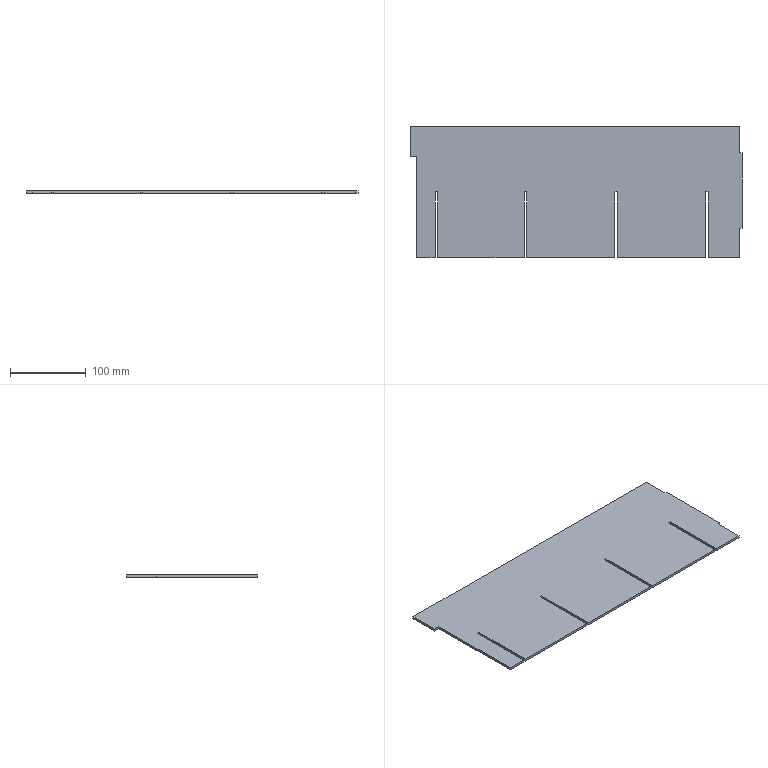Part | SolidWorks | features FlatPattern 1, SMBaseFlange 1, SheetMetal 1 | 1 solid | 28 faces | box 439 x 173.7 x 3.2 mm | volume 236184 mm3 | plane 28
STEP:
#1=CARTESIAN_POINT('',(-218.,59.63,0.));
#2=VERTEX_POINT('',#1);
#3=CARTESIAN_POINT('',(-654.,59.63,0.));
#4=VERTEX_POINT('',#3);
#5=CARTESIAN_POINT('',(-218.,59.63,0.));
#6=DIRECTION('',(-1.,0.,0.));
#7=VECTOR('',#6,1000.);
#8=LINE('',#5,#7);
#9=EDGE_CURVE('',#2,#4,#8,.T.);
#10=ORIENTED_EDGE('',*,*,#9,.T.);
#11=CARTESIAN_POINT('',(-654.,59.63,3.2));
#12=VERTEX_POINT('',#11);
#13=CARTESIAN_POINT('',(-654.,59.63,3.2));
#14=DIRECTION('',(0.,0.,-1.));
#15=VECTOR('',#14,1000.);
#16=LINE('',#13,#15);
#17=EDGE_CURVE('',#12,#4,#16,.T.);
#18=ORIENTED_EDGE('',*,*,#17,.F.);
#19=CARTESIAN_POINT('',(-218.,59.63,3.2));
#20=VERTEX_POINT('',#19);
#21=CARTESIAN_POINT('',(-218.,59.63,3.2));
#22=DIRECTION('',(-1.,0.,0.));
#23=VECTOR('',#22,1000.);
#24=LINE('',#21,#23);
#25=EDGE_CURVE('',#20,#12,#24,.T.);
#26=ORIENTED_EDGE('',*,*,#25,.F.);
#27=CARTESIAN_POINT('',(-218.,59.63,3.2));
#28=DIRECTION('',(0.,0.,-1.));
#29=VECTOR('',#28,1000.);
#30=LINE('',#27,#29);
#31=EDGE_CURVE('',#20,#2,#30,.T.);
#32=ORIENTED_EDGE('',*,*,#31,.T.);
#33=EDGE_LOOP('',(#10,#18,#26,#32));
#34=FACE_OUTER_BOUND('',#33,.T.);
#35=CARTESIAN_POINT('',(-218.,59.63,3.2));
#36=DIRECTION('',(0.,-1.,0.));
#37=DIRECTION('',(0.,0.,-1.));
#38=AXIS2_PLACEMENT_3D('',#35,#36,#37);
#39=PLANE('',#38);
#40=ADVANCED_FACE('',(#34),#39,.F.);
#41=CARTESIAN_POINT('',(-654.,19.93,0.));
#42=VERTEX_POINT('',#41);
#43=CARTESIAN_POINT('',(-654.,59.63,0.));
#44=DIRECTION('',(0.,-1.,0.));
#45=VECTOR('',#44,1000.);
#46=LINE('',#43,#45);
#47=EDGE_CURVE('',#4,#42,#46,.T.);
#48=ORIENTED_EDGE('',*,*,#47,.T.);
#49=CARTESIAN_POINT('',(-654.,19.93,3.2));
#50=VERTEX_POINT('',#49);
#51=CARTESIAN_POINT('',(-654.,19.93,3.2));
#52=DIRECTION('',(0.,0.,-1.));
#53=VECTOR('',#52,1000.);
#54=LINE('',#51,#53);
#55=EDGE_CURVE('',#50,#42,#54,.T.);
#56=ORIENTED_EDGE('',*,*,#55,.F.);
#57=CARTESIAN_POINT('',(-654.,59.63,3.2));
#58=DIRECTION('',(0.,-1.,0.));
#59=VECTOR('',#58,1000.);
#60=LINE('',#57,#59);
#61=EDGE_CURVE('',#12,#50,#60,.T.);
#62=ORIENTED_EDGE('',*,*,#61,.F.);
#63=ORIENTED_EDGE('',*,*,#17,.T.);
#64=EDGE_LOOP('',(#48,#56,#62,#63));
#65=FACE_OUTER_BOUND('',#64,.T.);
#66=CARTESIAN_POINT('',(-654.,59.63,3.2));
#67=DIRECTION('',(1.,0.,0.));
#68=DIRECTION('',(0.,0.,-1.));
#69=AXIS2_PLACEMENT_3D('',#66,#67,#68);
#70=PLANE('',#69);
#71=ADVANCED_FACE('',(#65),#70,.F.);
#72=CARTESIAN_POINT('',(-645.7,19.93,0.));
#73=VERTEX_POINT('',#72);
#74=CARTESIAN_POINT('',(-654.,19.93,0.));
#75=DIRECTION('',(1.,0.,0.));
#76=VECTOR('',#75,1000.);
#77=LINE('',#74,#76);
#78=EDGE_CURVE('',#42,#73,#77,.T.);
#79=ORIENTED_EDGE('',*,*,#78,.T.);
#80=CARTESIAN_POINT('',(-645.7,19.93,3.2));
#81=VERTEX_POINT('',#80);
#82=CARTESIAN_POINT('',(-645.7,19.93,3.2));
#83=DIRECTION('',(0.,0.,-1.));
#84=VECTOR('',#83,1000.);
#85=LINE('',#82,#84);
#86=EDGE_CURVE('',#81,#73,#85,.T.);
#87=ORIENTED_EDGE('',*,*,#86,.F.);
#88=CARTESIAN_POINT('',(-654.,19.93,3.2));
#89=DIRECTION('',(1.,0.,0.));
#90=VECTOR('',#89,1000.);
#91=LINE('',#88,#90);
#92=EDGE_CURVE('',#50,#81,#91,.T.);
#93=ORIENTED_EDGE('',*,*,#92,.F.);
#94=ORIENTED_EDGE('',*,*,#55,.T.);
#95=EDGE_LOOP('',(#79,#87,#93,#94));
#96=FACE_OUTER_BOUND('',#95,.T.);
#97=CARTESIAN_POINT('',(-654.,19.93,3.2));
#98=DIRECTION('',(0.,1.,0.));
#99=DIRECTION('',(0.,0.,1.));
#100=AXIS2_PLACEMENT_3D('',#97,#98,#99);
#101=PLANE('',#100);
#102=ADVANCED_FACE('',(#96),#101,.F.);
#103=CARTESIAN_POINT('',(-645.7,-114.07,0.));
#104=VERTEX_POINT('',#103);
#105=CARTESIAN_POINT('',(-645.7,19.93,0.));
#106=DIRECTION('',(0.,-1.,0.));
#107=VECTOR('',#106,1000.);
#108=LINE('',#105,#107);
#109=EDGE_CURVE('',#73,#104,#108,.T.);
#110=ORIENTED_EDGE('',*,*,#109,.T.);
#111=CARTESIAN_POINT('',(-645.7,-114.07,3.2));
#112=VERTEX_POINT('',#111);
#113=CARTESIAN_POINT('',(-645.7,-114.07,3.2));
#114=DIRECTION('',(0.,0.,-1.));
#115=VECTOR('',#114,1000.);
#116=LINE('',#113,#115);
#117=EDGE_CURVE('',#112,#104,#116,.T.);
#118=ORIENTED_EDGE('',*,*,#117,.F.);
#119=CARTESIAN_POINT('',(-645.7,19.93,3.2));
#120=DIRECTION('',(0.,-1.,0.));
#121=VECTOR('',#120,1000.);
#122=LINE('',#119,#121);
#123=EDGE_CURVE('',#81,#112,#122,.T.);
#124=ORIENTED_EDGE('',*,*,#123,.F.);
#125=ORIENTED_EDGE('',*,*,#86,.T.);
#126=EDGE_LOOP('',(#110,#118,#124,#125));
#127=FACE_OUTER_BOUND('',#126,.T.);
#128=CARTESIAN_POINT('',(-645.7,19.93,3.2));
#129=DIRECTION('',(1.,0.,0.));
#130=DIRECTION('',(0.,1.,0.));
#131=AXIS2_PLACEMENT_3D('',#128,#129,#130);
#132=PLANE('',#131);
#133=ADVANCED_FACE('',(#127),#132,.F.);
#134=CARTESIAN_POINT('',(-620.7,-114.07,0.));
#135=VERTEX_POINT('',#134);
#136=CARTESIAN_POINT('',(-645.7,-114.07,0.));
#137=DIRECTION('',(1.,0.,0.));
#138=VECTOR('',#137,1000.);
#139=LINE('',#136,#138);
#140=EDGE_CURVE('',#104,#135,#139,.T.);
#141=ORIENTED_EDGE('',*,*,#140,.T.);
#142=CARTESIAN_POINT('',(-620.7,-114.07,3.2));
#143=VERTEX_POINT('',#142);
#144=CARTESIAN_POINT('',(-620.7,-114.07,3.2));
#145=DIRECTION('',(0.,0.,-1.));
#146=VECTOR('',#145,1000.);
#147=LINE('',#144,#146);
#148=EDGE_CURVE('',#143,#135,#147,.T.);
#149=ORIENTED_EDGE('',*,*,#148,.F.);
#150=CARTESIAN_POINT('',(-645.7,-114.07,3.2));
#151=DIRECTION('',(1.,0.,0.));
#152=VECTOR('',#151,1000.);
#153=LINE('',#150,#152);
#154=EDGE_CURVE('',#112,#143,#153,.T.);
#155=ORIENTED_EDGE('',*,*,#154,.F.);
#156=ORIENTED_EDGE('',*,*,#117,.T.);
#157=EDGE_LOOP('',(#141,#149,#155,#156));
#158=FACE_OUTER_BOUND('',#157,.T.);
#159=CARTESIAN_POINT('',(-645.7,-114.07,3.2));
#160=DIRECTION('',(0.,1.,0.));
#161=DIRECTION('',(-1.,0.,0.));
#162=AXIS2_PLACEMENT_3D('',#159,#160,#161);
#163=PLANE('',#162);
#164=ADVANCED_FACE('',(#158),#163,.F.);
#165=CARTESIAN_POINT('',(-620.7,-27.07,0.));
#166=VERTEX_POINT('',#165);
#167=CARTESIAN_POINT('',(-620.7,-114.07,0.));
#168=DIRECTION('',(0.,1.,0.));
#169=VECTOR('',#168,1000.);
#170=LINE('',#167,#169);
#171=EDGE_CURVE('',#135,#166,#170,.T.);
#172=ORIENTED_EDGE('',*,*,#171,.T.);
#173=CARTESIAN_POINT('',(-620.7,-27.07,3.2));
#174=VERTEX_POINT('',#173);
#175=CARTESIAN_POINT('',(-620.7,-27.07,3.2));
#176=DIRECTION('',(0.,0.,-1.));
#177=VECTOR('',#176,1000.);
#178=LINE('',#175,#177);
#179=EDGE_CURVE('',#174,#166,#178,.T.);
#180=ORIENTED_EDGE('',*,*,#179,.F.);
#181=CARTESIAN_POINT('',(-620.7,-114.07,3.2));
#182=DIRECTION('',(0.,1.,0.));
#183=VECTOR('',#182,1000.);
#184=LINE('',#181,#183);
#185=EDGE_CURVE('',#143,#174,#184,.T.);
#186=ORIENTED_EDGE('',*,*,#185,.F.);
#187=ORIENTED_EDGE('',*,*,#148,.T.);
#188=EDGE_LOOP('',(#172,#180,#186,#187));
#189=FACE_OUTER_BOUND('',#188,.T.);
#190=CARTESIAN_POINT('',(-620.7,-114.07,3.2));
#191=DIRECTION('',(-1.,0.,0.));
#192=DIRECTION('',(0.,-1.,0.));
#193=AXIS2_PLACEMENT_3D('',#190,#191,#192);
#194=PLANE('',#193);
#195=ADVANCED_FACE('',(#189),#194,.F.);
#196=CARTESIAN_POINT('',(-617.5,-27.07,0.));
#197=VERTEX_POINT('',#196);
#198=CARTESIAN_POINT('',(-620.7,-27.07,0.));
#199=DIRECTION('',(1.,0.,0.));
#200=VECTOR('',#199,1000.);
#201=LINE('',#198,#200);
#202=EDGE_CURVE('',#166,#197,#201,.T.);
#203=ORIENTED_EDGE('',*,*,#202,.T.);
#204=CARTESIAN_POINT('',(-617.5,-27.07,3.2));
#205=VERTEX_POINT('',#204);
#206=CARTESIAN_POINT('',(-617.5,-27.07,3.2));
#207=DIRECTION('',(0.,0.,-1.));
#208=VECTOR('',#207,1000.);
#209=LINE('',#206,#208);
#210=EDGE_CURVE('',#205,#197,#209,.T.);
#211=ORIENTED_EDGE('',*,*,#210,.F.);
#212=CARTESIAN_POINT('',(-620.7,-27.07,3.2));
#213=DIRECTION('',(1.,0.,0.));
#214=VECTOR('',#213,1000.);
#215=LINE('',#212,#214);
#216=EDGE_CURVE('',#174,#205,#215,.T.);
#217=ORIENTED_EDGE('',*,*,#216,.F.);
#218=ORIENTED_EDGE('',*,*,#179,.T.);
#219=EDGE_LOOP('',(#203,#211,#217,#218));
#220=FACE_OUTER_BOUND('',#219,.T.);
#221=CARTESIAN_POINT('',(-620.7,-27.07,3.2));
#222=DIRECTION('',(0.,1.,0.));
#223=DIRECTION('',(0.,0.,1.));
#224=AXIS2_PLACEMENT_3D('',#221,#222,#223);
#225=PLANE('',#224);
#226=ADVANCED_FACE('',(#220),#225,.F.);
#227=CARTESIAN_POINT('',(-617.5,-114.07,0.));
#228=VERTEX_POINT('',#227);
#229=CARTESIAN_POINT('',(-617.5,-27.07,0.));
#230=DIRECTION('',(0.,-1.,0.));
#231=VECTOR('',#230,1000.);
#232=LINE('',#229,#231);
#233=EDGE_CURVE('',#197,#228,#232,.T.);
#234=ORIENTED_EDGE('',*,*,#233,.T.);
#235=CARTESIAN_POINT('',(-617.5,-114.07,3.2));
#236=VERTEX_POINT('',#235);
#237=CARTESIAN_POINT('',(-617.5,-114.07,3.2));
#238=DIRECTION('',(0.,0.,-1.));
#239=VECTOR('',#238,1000.);
#240=LINE('',#237,#239);
#241=EDGE_CURVE('',#236,#228,#240,.T.);
#242=ORIENTED_EDGE('',*,*,#241,.F.);
#243=CARTESIAN_POINT('',(-617.5,-27.07,3.2));
#244=DIRECTION('',(0.,-1.,0.));
#245=VECTOR('',#244,1000.);
#246=LINE('',#243,#245);
#247=EDGE_CURVE('',#205,#236,#246,.T.);
#248=ORIENTED_EDGE('',*,*,#247,.F.);
#249=ORIENTED_EDGE('',*,*,#210,.T.);
#250=EDGE_LOOP('',(#234,#242,#248,#249));
#251=FACE_OUTER_BOUND('',#250,.T.);
#252=CARTESIAN_POINT('',(-617.5,-27.07,3.2));
#253=DIRECTION('',(1.,0.,0.));
#254=DIRECTION('',(0.,1.,0.));
#255=AXIS2_PLACEMENT_3D('',#252,#253,#254);
#256=PLANE('',#255);
#257=ADVANCED_FACE('',(#251),#256,.F.);
#258=CARTESIAN_POINT('',(-503.,-114.07,0.));
#259=VERTEX_POINT('',#258);
#260=CARTESIAN_POINT('',(-617.5,-114.07,0.));
#261=DIRECTION('',(1.,0.,0.));
#262=VECTOR('',#261,1000.);
#263=LINE('',#260,#262);
#264=EDGE_CURVE('',#228,#259,#263,.T.);
#265=ORIENTED_EDGE('',*,*,#264,.T.);
#266=CARTESIAN_POINT('',(-503.,-114.07,3.2));
#267=VERTEX_POINT('',#266);
#268=CARTESIAN_POINT('',(-503.,-114.07,3.2));
#269=DIRECTION('',(0.,0.,-1.));
#270=VECTOR('',#269,1000.);
#271=LINE('',#268,#270);
#272=EDGE_CURVE('',#267,#259,#271,.T.);
#273=ORIENTED_EDGE('',*,*,#272,.F.);
#274=CARTESIAN_POINT('',(-617.5,-114.07,3.2));
#275=DIRECTION('',(1.,0.,0.));
#276=VECTOR('',#275,1000.);
#277=LINE('',#274,#276);
#278=EDGE_CURVE('',#236,#267,#277,.T.);
#279=ORIENTED_EDGE('',*,*,#278,.F.);
#280=ORIENTED_EDGE('',*,*,#241,.T.);
#281=EDGE_LOOP('',(#265,#273,#279,#280));
#282=FACE_OUTER_BOUND('',#281,.T.);
#283=CARTESIAN_POINT('',(-617.5,-114.07,3.2));
#284=DIRECTION('',(0.,1.,0.));
#285=DIRECTION('',(0.,0.,1.));
#286=AXIS2_PLACEMENT_3D('',#283,#284,#285);
#287=PLANE('',#286);
#288=ADVANCED_FACE('',(#282),#287,.F.);
#289=CARTESIAN_POINT('',(-503.,-27.07,0.));
#290=VERTEX_POINT('',#289);
#291=CARTESIAN_POINT('',(-503.,-114.07,0.));
#292=DIRECTION('',(0.,1.,0.));
#293=VECTOR('',#292,1000.);
#294=LINE('',#291,#293);
#295=EDGE_CURVE('',#259,#290,#294,.T.);
#296=ORIENTED_EDGE('',*,*,#295,.T.);
#297=CARTESIAN_POINT('',(-503.,-27.07,3.2));
#298=VERTEX_POINT('',#297);
#299=CARTESIAN_POINT('',(-503.,-27.07,3.2));
#300=DIRECTION('',(0.,0.,-1.));
#301=VECTOR('',#300,1000.);
#302=LINE('',#299,#301);
#303=EDGE_CURVE('',#298,#290,#302,.T.);
#304=ORIENTED_EDGE('',*,*,#303,.F.);
#305=CARTESIAN_POINT('',(-503.,-114.07,3.2));
#306=DIRECTION('',(0.,1.,0.));
#307=VECTOR('',#306,1000.);
#308=LINE('',#305,#307);
#309=EDGE_CURVE('',#267,#298,#308,.T.);
#310=ORIENTED_EDGE('',*,*,#309,.F.);
#311=ORIENTED_EDGE('',*,*,#272,.T.);
#312=EDGE_LOOP('',(#296,#304,#310,#311));
#313=FACE_OUTER_BOUND('',#312,.T.);
#314=CARTESIAN_POINT('',(-503.,-114.07,3.2));
#315=DIRECTION('',(-1.,0.,0.));
#316=DIRECTION('',(0.,0.,1.));
#317=AXIS2_PLACEMENT_3D('',#314,#315,#316);
#318=PLANE('',#317);
#319=ADVANCED_FACE('',(#313),#318,.F.);
#320=CARTESIAN_POINT('',(-499.8,-27.07,0.));
#321=VERTEX_POINT('',#320);
#322=CARTESIAN_POINT('',(-503.,-27.07,0.));
#323=DIRECTION('',(1.,0.,0.));
#324=VECTOR('',#323,1000.);
#325=LINE('',#322,#324);
#326=EDGE_CURVE('',#290,#321,#325,.T.);
#327=ORIENTED_EDGE('',*,*,#326,.T.);
#328=CARTESIAN_POINT('',(-499.8,-27.07,3.2));
#329=VERTEX_POINT('',#328);
#330=CARTESIAN_POINT('',(-499.8,-27.07,3.2));
#331=DIRECTION('',(0.,0.,-1.));
#332=VECTOR('',#331,1000.);
#333=LINE('',#330,#332);
#334=EDGE_CURVE('',#329,#321,#333,.T.);
#335=ORIENTED_EDGE('',*,*,#334,.F.);
#336=CARTESIAN_POINT('',(-503.,-27.07,3.2));
#337=DIRECTION('',(1.,0.,0.));
#338=VECTOR('',#337,1000.);
#339=LINE('',#336,#338);
#340=EDGE_CURVE('',#298,#329,#339,.T.);
#341=ORIENTED_EDGE('',*,*,#340,.F.);
#342=ORIENTED_EDGE('',*,*,#303,.T.);
#343=EDGE_LOOP('',(#327,#335,#341,#342));
#344=FACE_OUTER_BOUND('',#343,.T.);
#345=CARTESIAN_POINT('',(-503.,-27.07,3.2));
#346=DIRECTION('',(0.,1.,0.));
#347=DIRECTION('',(0.,0.,1.));
#348=AXIS2_PLACEMENT_3D('',#345,#346,#347);
#349=PLANE('',#348);
#350=ADVANCED_FACE('',(#344),#349,.F.);
#351=CARTESIAN_POINT('',(-499.8,-114.07,0.));
#352=VERTEX_POINT('',#351);
#353=CARTESIAN_POINT('',(-499.8,-27.07,0.));
#354=DIRECTION('',(0.,-1.,0.));
#355=VECTOR('',#354,1000.);
#356=LINE('',#353,#355);
#357=EDGE_CURVE('',#321,#352,#356,.T.);
#358=ORIENTED_EDGE('',*,*,#357,.T.);
#359=CARTESIAN_POINT('',(-499.8,-114.07,3.2));
#360=VERTEX_POINT('',#359);
#361=CARTESIAN_POINT('',(-499.8,-114.07,3.2));
#362=DIRECTION('',(0.,0.,-1.));
#363=VECTOR('',#362,1000.);
#364=LINE('',#361,#363);
#365=EDGE_CURVE('',#360,#352,#364,.T.);
#366=ORIENTED_EDGE('',*,*,#365,.F.);
#367=CARTESIAN_POINT('',(-499.8,-27.07,3.2));
#368=DIRECTION('',(0.,-1.,0.));
#369=VECTOR('',#368,1000.);
#370=LINE('',#367,#369);
#371=EDGE_CURVE('',#329,#360,#370,.T.);
#372=ORIENTED_EDGE('',*,*,#371,.F.);
#373=ORIENTED_EDGE('',*,*,#334,.T.);
#374=EDGE_LOOP('',(#358,#366,#372,#373));
#375=FACE_OUTER_BOUND('',#374,.T.);
#376=CARTESIAN_POINT('',(-499.8,-27.07,3.2));
#377=DIRECTION('',(1.,0.,0.));
#378=DIRECTION('',(0.,0.,-1.));
#379=AXIS2_PLACEMENT_3D('',#376,#377,#378);
#380=PLANE('',#379);
#381=ADVANCED_FACE('',(#375),#380,.F.);
#382=CARTESIAN_POINT('',(-383.,-114.07,0.));
#383=VERTEX_POINT('',#382);
#384=CARTESIAN_POINT('',(-499.8,-114.07,0.));
#385=DIRECTION('',(1.,0.,0.));
#386=VECTOR('',#385,1000.);
#387=LINE('',#384,#386);
#388=EDGE_CURVE('',#352,#383,#387,.T.);
#389=ORIENTED_EDGE('',*,*,#388,.T.);
#390=CARTESIAN_POINT('',(-383.,-114.07,3.2));
#391=VERTEX_POINT('',#390);
#392=CARTESIAN_POINT('',(-383.,-114.07,3.2));
#393=DIRECTION('',(0.,0.,-1.));
#394=VECTOR('',#393,1000.);
#395=LINE('',#392,#394);
#396=EDGE_CURVE('',#391,#383,#395,.T.);
#397=ORIENTED_EDGE('',*,*,#396,.F.);
#398=CARTESIAN_POINT('',(-499.8,-114.07,3.2));
#399=DIRECTION('',(1.,0.,0.));
#400=VECTOR('',#399,1000.);
#401=LINE('',#398,#400);
#402=EDGE_CURVE('',#360,#391,#401,.T.);
#403=ORIENTED_EDGE('',*,*,#402,.F.);
#404=ORIENTED_EDGE('',*,*,#365,.T.);
#405=EDGE_LOOP('',(#389,#397,#403,#404));
#406=FACE_OUTER_BOUND('',#405,.T.);
#407=CARTESIAN_POINT('',(-499.8,-114.07,3.2));
#408=DIRECTION('',(0.,1.,0.));
#409=DIRECTION('',(0.,0.,1.));
#410=AXIS2_PLACEMENT_3D('',#407,#408,#409);
#411=PLANE('',#410);
#412=ADVANCED_FACE('',(#406),#411,.F.);
#413=CARTESIAN_POINT('',(-383.,-27.07,0.));
#414=VERTEX_POINT('',#413);
#415=CARTESIAN_POINT('',(-383.,-114.07,0.));
#416=DIRECTION('',(0.,1.,0.));
#417=VECTOR('',#416,1000.);
#418=LINE('',#415,#417);
#419=EDGE_CURVE('',#383,#414,#418,.T.);
#420=ORIENTED_EDGE('',*,*,#419,.T.);
#421=CARTESIAN_POINT('',(-383.,-27.07,3.2));
#422=VERTEX_POINT('',#421);
#423=CARTESIAN_POINT('',(-383.,-27.07,3.2));
#424=DIRECTION('',(0.,0.,-1.));
#425=VECTOR('',#424,1000.);
#426=LINE('',#423,#425);
#427=EDGE_CURVE('',#422,#414,#426,.T.);
#428=ORIENTED_EDGE('',*,*,#427,.F.);
#429=CARTESIAN_POINT('',(-383.,-114.07,3.2));
#430=DIRECTION('',(0.,1.,0.));
#431=VECTOR('',#430,1000.);
#432=LINE('',#429,#431);
#433=EDGE_CURVE('',#391,#422,#432,.T.);
#434=ORIENTED_EDGE('',*,*,#433,.F.);
#435=ORIENTED_EDGE('',*,*,#396,.T.);
#436=EDGE_LOOP('',(#420,#428,#434,#435));
#437=FACE_OUTER_BOUND('',#436,.T.);
#438=CARTESIAN_POINT('',(-383.,-114.07,3.2));
#439=DIRECTION('',(-1.,0.,0.));
#440=DIRECTION('',(0.,0.,1.));
#441=AXIS2_PLACEMENT_3D('',#438,#439,#440);
#442=PLANE('',#441);
#443=ADVANCED_FACE('',(#437),#442,.F.);
#444=CARTESIAN_POINT('',(-379.8,-27.07,0.));
#445=VERTEX_POINT('',#444);
#446=CARTESIAN_POINT('',(-383.,-27.07,0.));
#447=DIRECTION('',(1.,0.,0.));
#448=VECTOR('',#447,1000.);
#449=LINE('',#446,#448);
#450=EDGE_CURVE('',#414,#445,#449,.T.);
#451=ORIENTED_EDGE('',*,*,#450,.T.);
#452=CARTESIAN_POINT('',(-379.8,-27.07,3.2));
#453=VERTEX_POINT('',#452);
#454=CARTESIAN_POINT('',(-379.8,-27.07,3.2));
#455=DIRECTION('',(0.,0.,-1.));
#456=VECTOR('',#455,1000.);
#457=LINE('',#454,#456);
#458=EDGE_CURVE('',#453,#445,#457,.T.);
#459=ORIENTED_EDGE('',*,*,#458,.F.);
#460=CARTESIAN_POINT('',(-383.,-27.07,3.2));
#461=DIRECTION('',(1.,0.,0.));
#462=VECTOR('',#461,1000.);
#463=LINE('',#460,#462);
#464=EDGE_CURVE('',#422,#453,#463,.T.);
#465=ORIENTED_EDGE('',*,*,#464,.F.);
#466=ORIENTED_EDGE('',*,*,#427,.T.);
#467=EDGE_LOOP('',(#451,#459,#465,#466));
#468=FACE_OUTER_BOUND('',#467,.T.);
#469=CARTESIAN_POINT('',(-383.,-27.07,3.2));
#470=DIRECTION('',(0.,1.,0.));
#471=DIRECTION('',(0.,0.,1.));
#472=AXIS2_PLACEMENT_3D('',#469,#470,#471);
#473=PLANE('',#472);
#474=ADVANCED_FACE('',(#468),#473,.F.);
#475=CARTESIAN_POINT('',(-379.8,-114.07,0.));
#476=VERTEX_POINT('',#475);
#477=CARTESIAN_POINT('',(-379.8,-27.07,0.));
#478=DIRECTION('',(0.,-1.,0.));
#479=VECTOR('',#478,1000.);
#480=LINE('',#477,#479);
#481=EDGE_CURVE('',#445,#476,#480,.T.);
#482=ORIENTED_EDGE('',*,*,#481,.T.);
#483=CARTESIAN_POINT('',(-379.8,-114.07,3.2));
#484=VERTEX_POINT('',#483);
#485=CARTESIAN_POINT('',(-379.8,-114.07,3.2));
#486=DIRECTION('',(0.,0.,-1.));
#487=VECTOR('',#486,1000.);
#488=LINE('',#485,#487);
#489=EDGE_CURVE('',#484,#476,#488,.T.);
#490=ORIENTED_EDGE('',*,*,#489,.F.);
#491=CARTESIAN_POINT('',(-379.8,-27.07,3.2));
#492=DIRECTION('',(0.,-1.,0.));
#493=VECTOR('',#492,1000.);
#494=LINE('',#491,#493);
#495=EDGE_CURVE('',#453,#484,#494,.T.);
#496=ORIENTED_EDGE('',*,*,#495,.F.);
#497=ORIENTED_EDGE('',*,*,#458,.T.);
#498=EDGE_LOOP('',(#482,#490,#496,#497));
#499=FACE_OUTER_BOUND('',#498,.T.);
#500=CARTESIAN_POINT('',(-379.8,-27.07,3.2));
#501=DIRECTION('',(1.,0.,0.));
#502=DIRECTION('',(0.,0.,-1.));
#503=AXIS2_PLACEMENT_3D('',#500,#501,#502);
#504=PLANE('',#503);
#505=ADVANCED_FACE('',(#499),#504,.F.);
#506=CARTESIAN_POINT('',(-263.,-114.07,0.));
#507=VERTEX_POINT('',#506);
#508=CARTESIAN_POINT('',(-379.8,-114.07,0.));
#509=DIRECTION('',(1.,0.,0.));
#510=VECTOR('',#509,1000.);
#511=LINE('',#508,#510);
#512=EDGE_CURVE('',#476,#507,#511,.T.);
#513=ORIENTED_EDGE('',*,*,#512,.T.);
#514=CARTESIAN_POINT('',(-263.,-114.07,3.2));
#515=VERTEX_POINT('',#514);
#516=CARTESIAN_POINT('',(-263.,-114.07,3.2));
#517=DIRECTION('',(0.,0.,-1.));
#518=VECTOR('',#517,1000.);
#519=LINE('',#516,#518);
#520=EDGE_CURVE('',#515,#507,#519,.T.);
#521=ORIENTED_EDGE('',*,*,#520,.F.);
#522=CARTESIAN_POINT('',(-379.8,-114.07,3.2));
#523=DIRECTION('',(1.,0.,0.));
#524=VECTOR('',#523,1000.);
#525=LINE('',#522,#524);
#526=EDGE_CURVE('',#484,#515,#525,.T.);
#527=ORIENTED_EDGE('',*,*,#526,.F.);
#528=ORIENTED_EDGE('',*,*,#489,.T.);
#529=EDGE_LOOP('',(#513,#521,#527,#528));
#530=FACE_OUTER_BOUND('',#529,.T.);
#531=CARTESIAN_POINT('',(-379.8,-114.07,3.2));
#532=DIRECTION('',(0.,1.,0.));
#533=DIRECTION('',(0.,0.,1.));
#534=AXIS2_PLACEMENT_3D('',#531,#532,#533);
#535=PLANE('',#534);
#536=ADVANCED_FACE('',(#530),#535,.F.);
#537=CARTESIAN_POINT('',(-263.,-27.07,0.));
#538=VERTEX_POINT('',#537);
#539=CARTESIAN_POINT('',(-263.,-114.07,0.));
#540=DIRECTION('',(0.,1.,0.));
#541=VECTOR('',#540,1000.);
#542=LINE('',#539,#541);
#543=EDGE_CURVE('',#507,#538,#542,.T.);
#544=ORIENTED_EDGE('',*,*,#543,.T.);
#545=CARTESIAN_POINT('',(-263.,-27.07,3.2));
#546=VERTEX_POINT('',#545);
#547=CARTESIAN_POINT('',(-263.,-27.07,3.2));
#548=DIRECTION('',(0.,0.,-1.));
#549=VECTOR('',#548,1000.);
#550=LINE('',#547,#549);
#551=EDGE_CURVE('',#546,#538,#550,.T.);
#552=ORIENTED_EDGE('',*,*,#551,.F.);
#553=CARTESIAN_POINT('',(-263.,-114.07,3.2));
#554=DIRECTION('',(0.,1.,0.));
#555=VECTOR('',#554,1000.);
#556=LINE('',#553,#555);
#557=EDGE_CURVE('',#515,#546,#556,.T.);
#558=ORIENTED_EDGE('',*,*,#557,.F.);
#559=ORIENTED_EDGE('',*,*,#520,.T.);
#560=EDGE_LOOP('',(#544,#552,#558,#559));
#561=FACE_OUTER_BOUND('',#560,.T.);
#562=CARTESIAN_POINT('',(-263.,-114.07,3.2));
#563=DIRECTION('',(-1.,0.,0.));
#564=DIRECTION('',(0.,0.,1.));
#565=AXIS2_PLACEMENT_3D('',#562,#563,#564);
#566=PLANE('',#565);
#567=ADVANCED_FACE('',(#561),#566,.F.);
#568=CARTESIAN_POINT('',(-259.8,-27.07,0.));
#569=VERTEX_POINT('',#568);
#570=CARTESIAN_POINT('',(-263.,-27.07,0.));
#571=DIRECTION('',(1.,0.,0.));
#572=VECTOR('',#571,1000.);
#573=LINE('',#570,#572);
#574=EDGE_CURVE('',#538,#569,#573,.T.);
#575=ORIENTED_EDGE('',*,*,#574,.T.);
#576=CARTESIAN_POINT('',(-259.8,-27.07,3.2));
#577=VERTEX_POINT('',#576);
#578=CARTESIAN_POINT('',(-259.8,-27.07,3.2));
#579=DIRECTION('',(0.,0.,-1.));
#580=VECTOR('',#579,1000.);
#581=LINE('',#578,#580);
#582=EDGE_CURVE('',#577,#569,#581,.T.);
#583=ORIENTED_EDGE('',*,*,#582,.F.);
#584=CARTESIAN_POINT('',(-263.,-27.07,3.2));
#585=DIRECTION('',(1.,0.,0.));
#586=VECTOR('',#585,1000.);
#587=LINE('',#584,#586);
#588=EDGE_CURVE('',#546,#577,#587,.T.);
#589=ORIENTED_EDGE('',*,*,#588,.F.);
#590=ORIENTED_EDGE('',*,*,#551,.T.);
#591=EDGE_LOOP('',(#575,#583,#589,#590));
#592=FACE_OUTER_BOUND('',#591,.T.);
#593=CARTESIAN_POINT('',(-263.,-27.07,3.2));
#594=DIRECTION('',(0.,1.,0.));
#595=DIRECTION('',(0.,0.,1.));
#596=AXIS2_PLACEMENT_3D('',#593,#594,#595);
#597=PLANE('',#596);
#598=ADVANCED_FACE('',(#592),#597,.F.);
#599=CARTESIAN_POINT('',(-259.8,-114.07,0.));
#600=VERTEX_POINT('',#599);
#601=CARTESIAN_POINT('',(-259.8,-27.07,0.));
#602=DIRECTION('',(0.,-1.,0.));
#603=VECTOR('',#602,1000.);
#604=LINE('',#601,#603);
#605=EDGE_CURVE('',#569,#600,#604,.T.);
#606=ORIENTED_EDGE('',*,*,#605,.T.);
#607=CARTESIAN_POINT('',(-259.8,-114.07,3.2));
#608=VERTEX_POINT('',#607);
#609=CARTESIAN_POINT('',(-259.8,-114.07,3.2));
#610=DIRECTION('',(0.,0.,-1.));
#611=VECTOR('',#610,1000.);
#612=LINE('',#609,#611);
#613=EDGE_CURVE('',#608,#600,#612,.T.);
#614=ORIENTED_EDGE('',*,*,#613,.F.);
#615=CARTESIAN_POINT('',(-259.8,-27.07,3.2));
#616=DIRECTION('',(0.,-1.,0.));
#617=VECTOR('',#616,1000.);
#618=LINE('',#615,#617);
#619=EDGE_CURVE('',#577,#608,#618,.T.);
#620=ORIENTED_EDGE('',*,*,#619,.F.);
#621=ORIENTED_EDGE('',*,*,#582,.T.);
#622=EDGE_LOOP('',(#606,#614,#620,#621));
#623=FACE_OUTER_BOUND('',#622,.T.);
#624=CARTESIAN_POINT('',(-259.8,-27.07,3.2));
#625=DIRECTION('',(1.,0.,0.));
#626=DIRECTION('',(0.,0.,-1.));
#627=AXIS2_PLACEMENT_3D('',#624,#625,#626);
#628=PLANE('',#627);
#629=ADVANCED_FACE('',(#623),#628,.F.);
#630=CARTESIAN_POINT('',(-218.,-114.07,0.));
#631=VERTEX_POINT('',#630);
#632=CARTESIAN_POINT('',(-259.8,-114.07,0.));
#633=DIRECTION('',(1.,0.,0.));
#634=VECTOR('',#633,1000.);
#635=LINE('',#632,#634);
#636=EDGE_CURVE('',#600,#631,#635,.T.);
#637=ORIENTED_EDGE('',*,*,#636,.T.);
#638=CARTESIAN_POINT('',(-218.,-114.07,3.2));
#639=VERTEX_POINT('',#638);
#640=CARTESIAN_POINT('',(-218.,-114.07,3.2));
#641=DIRECTION('',(0.,0.,-1.));
#642=VECTOR('',#641,1000.);
#643=LINE('',#640,#642);
#644=EDGE_CURVE('',#639,#631,#643,.T.);
#645=ORIENTED_EDGE('',*,*,#644,.F.);
#646=CARTESIAN_POINT('',(-259.8,-114.07,3.2));
#647=DIRECTION('',(1.,0.,0.));
#648=VECTOR('',#647,1000.);
#649=LINE('',#646,#648);
#650=EDGE_CURVE('',#608,#639,#649,.T.);
#651=ORIENTED_EDGE('',*,*,#650,.F.);
#652=ORIENTED_EDGE('',*,*,#613,.T.);
#653=EDGE_LOOP('',(#637,#645,#651,#652));
#654=FACE_OUTER_BOUND('',#653,.T.);
#655=CARTESIAN_POINT('',(-259.8,-114.07,3.2));
#656=DIRECTION('',(0.,1.,0.));
#657=DIRECTION('',(-1.,0.,0.));
#658=AXIS2_PLACEMENT_3D('',#655,#656,#657);
#659=PLANE('',#658);
#660=ADVANCED_FACE('',(#654),#659,.F.);
#661=CARTESIAN_POINT('',(-218.,-75.37,0.));
#662=VERTEX_POINT('',#661);
#663=CARTESIAN_POINT('',(-218.,-114.07,0.));
#664=DIRECTION('',(0.,1.,0.));
#665=VECTOR('',#664,1000.);
#666=LINE('',#663,#665);
#667=EDGE_CURVE('',#631,#662,#666,.T.);
#668=ORIENTED_EDGE('',*,*,#667,.T.);
#669=CARTESIAN_POINT('',(-218.,-75.37,3.2));
#670=VERTEX_POINT('',#669);
#671=CARTESIAN_POINT('',(-218.,-75.37,3.2));
#672=DIRECTION('',(0.,0.,-1.));
#673=VECTOR('',#672,1000.);
#674=LINE('',#671,#673);
#675=EDGE_CURVE('',#670,#662,#674,.T.);
#676=ORIENTED_EDGE('',*,*,#675,.F.);
#677=CARTESIAN_POINT('',(-218.,-114.07,3.2));
#678=DIRECTION('',(0.,1.,0.));
#679=VECTOR('',#678,1000.);
#680=LINE('',#677,#679);
#681=EDGE_CURVE('',#639,#670,#680,.T.);
#682=ORIENTED_EDGE('',*,*,#681,.F.);
#683=ORIENTED_EDGE('',*,*,#644,.T.);
#684=EDGE_LOOP('',(#668,#676,#682,#683));
#685=FACE_OUTER_BOUND('',#684,.T.);
#686=CARTESIAN_POINT('',(-218.,-114.07,3.2));
#687=DIRECTION('',(-1.,0.,0.));
#688=DIRECTION('',(0.,0.,1.));
#689=AXIS2_PLACEMENT_3D('',#686,#687,#688);
#690=PLANE('',#689);
#691=ADVANCED_FACE('',(#685),#690,.F.);
#692=CARTESIAN_POINT('',(-215.,-75.37,0.));
#693=VERTEX_POINT('',#692);
#694=CARTESIAN_POINT('',(-215.,-75.37,0.));
#695=DIRECTION('',(1.,0.,0.));
#696=VECTOR('',#695,1000.);
#697=LINE('',#694,#696);
#698=EDGE_CURVE('',#662,#693,#697,.T.);
#699=ORIENTED_EDGE('',*,*,#698,.T.);
#700=CARTESIAN_POINT('',(-215.,-75.37,3.2));
#701=VERTEX_POINT('',#700);
#702=CARTESIAN_POINT('',(-215.,-75.37,3.2));
#703=DIRECTION('',(0.,0.,-1.));
#704=VECTOR('',#703,1000.);
#705=LINE('',#702,#704);
#706=EDGE_CURVE('',#701,#693,#705,.T.);
#707=ORIENTED_EDGE('',*,*,#706,.F.);
#708=CARTESIAN_POINT('',(-215.,-75.37,3.2));
#709=DIRECTION('',(1.,0.,0.));
#710=VECTOR('',#709,1000.);
#711=LINE('',#708,#710);
#712=EDGE_CURVE('',#670,#701,#711,.T.);
#713=ORIENTED_EDGE('',*,*,#712,.F.);
#714=ORIENTED_EDGE('',*,*,#675,.T.);
#715=EDGE_LOOP('',(#699,#707,#713,#714));
#716=FACE_OUTER_BOUND('',#715,.T.);
#717=CARTESIAN_POINT('',(-215.,-75.37,3.2));
#718=DIRECTION('',(0.,1.,0.));
#719=DIRECTION('',(-1.,0.,0.));
#720=AXIS2_PLACEMENT_3D('',#717,#718,#719);
#721=PLANE('',#720);
#722=ADVANCED_FACE('',(#716),#721,.F.);
#723=CARTESIAN_POINT('',(-215.,24.63,0.));
#724=VERTEX_POINT('',#723);
#725=CARTESIAN_POINT('',(-215.,24.63,0.));
#726=DIRECTION('',(0.,1.,0.));
#727=VECTOR('',#726,1000.);
#728=LINE('',#725,#727);
#729=EDGE_CURVE('',#693,#724,#728,.T.);
#730=ORIENTED_EDGE('',*,*,#729,.T.);
#731=CARTESIAN_POINT('',(-215.,24.63,3.2));
#732=VERTEX_POINT('',#731);
#733=CARTESIAN_POINT('',(-215.,24.63,3.2));
#734=DIRECTION('',(0.,0.,-1.));
#735=VECTOR('',#734,1000.);
#736=LINE('',#733,#735);
#737=EDGE_CURVE('',#732,#724,#736,.T.);
#738=ORIENTED_EDGE('',*,*,#737,.F.);
#739=CARTESIAN_POINT('',(-215.,24.63,3.2));
#740=DIRECTION('',(0.,1.,0.));
#741=VECTOR('',#740,1000.);
#742=LINE('',#739,#741);
#743=EDGE_CURVE('',#701,#732,#742,.T.);
#744=ORIENTED_EDGE('',*,*,#743,.F.);
#745=ORIENTED_EDGE('',*,*,#706,.T.);
#746=EDGE_LOOP('',(#730,#738,#744,#745));
#747=FACE_OUTER_BOUND('',#746,.T.);
#748=CARTESIAN_POINT('',(-215.,24.63,3.2));
#749=DIRECTION('',(-1.,0.,0.));
#750=DIRECTION('',(0.,0.,1.));
#751=AXIS2_PLACEMENT_3D('',#748,#749,#750);
#752=PLANE('',#751);
#753=ADVANCED_FACE('',(#747),#752,.F.);
#754=CARTESIAN_POINT('',(-218.,24.63,0.));
#755=VERTEX_POINT('',#754);
#756=CARTESIAN_POINT('',(-218.,24.63,0.));
#757=DIRECTION('',(-1.,0.,0.));
#758=VECTOR('',#757,1000.);
#759=LINE('',#756,#758);
#760=EDGE_CURVE('',#724,#755,#759,.T.);
#761=ORIENTED_EDGE('',*,*,#760,.T.);
#762=CARTESIAN_POINT('',(-218.,24.63,3.2));
#763=VERTEX_POINT('',#762);
#764=CARTESIAN_POINT('',(-218.,24.63,3.2));
#765=DIRECTION('',(0.,0.,-1.));
#766=VECTOR('',#765,1000.);
#767=LINE('',#764,#766);
#768=EDGE_CURVE('',#763,#755,#767,.T.);
#769=ORIENTED_EDGE('',*,*,#768,.F.);
#770=CARTESIAN_POINT('',(-218.,24.63,3.2));
#771=DIRECTION('',(-1.,0.,0.));
#772=VECTOR('',#771,1000.);
#773=LINE('',#770,#772);
#774=EDGE_CURVE('',#732,#763,#773,.T.);
#775=ORIENTED_EDGE('',*,*,#774,.F.);
#776=ORIENTED_EDGE('',*,*,#737,.T.);
#777=EDGE_LOOP('',(#761,#769,#775,#776));
#778=FACE_OUTER_BOUND('',#777,.T.);
#779=CARTESIAN_POINT('',(-218.,24.63,3.2));
#780=DIRECTION('',(0.,-1.,0.));
#781=DIRECTION('',(0.,0.,-1.));
#782=AXIS2_PLACEMENT_3D('',#779,#780,#781);
#783=PLANE('',#782);
#784=ADVANCED_FACE('',(#778),#783,.F.);
#785=CARTESIAN_POINT('',(-218.,24.63,0.));
#786=DIRECTION('',(0.,1.,0.));
#787=VECTOR('',#786,1000.);
#788=LINE('',#785,#787);
#789=EDGE_CURVE('',#755,#2,#788,.T.);
#790=ORIENTED_EDGE('',*,*,#789,.T.);
#791=ORIENTED_EDGE('',*,*,#31,.F.);
#792=CARTESIAN_POINT('',(-218.,24.63,3.2));
#793=DIRECTION('',(0.,1.,0.));
#794=VECTOR('',#793,1000.);
#795=LINE('',#792,#794);
#796=EDGE_CURVE('',#763,#20,#795,.T.);
#797=ORIENTED_EDGE('',*,*,#796,.F.);
#798=ORIENTED_EDGE('',*,*,#768,.T.);
#799=EDGE_LOOP('',(#790,#791,#797,#798));
#800=FACE_OUTER_BOUND('',#799,.T.);
#801=CARTESIAN_POINT('',(-218.,24.63,3.2));
#802=DIRECTION('',(-1.,0.,0.));
#803=DIRECTION('',(0.,0.,1.));
#804=AXIS2_PLACEMENT_3D('',#801,#802,#803);
#805=PLANE('',#804);
#806=ADVANCED_FACE('',(#800),#805,.F.);
#807=ORIENTED_EDGE('',*,*,#25,.T.);
#808=ORIENTED_EDGE('',*,*,#61,.T.);
#809=ORIENTED_EDGE('',*,*,#92,.T.);
#810=ORIENTED_EDGE('',*,*,#123,.T.);
#811=ORIENTED_EDGE('',*,*,#154,.T.);
#812=ORIENTED_EDGE('',*,*,#185,.T.);
#813=ORIENTED_EDGE('',*,*,#216,.T.);
#814=ORIENTED_EDGE('',*,*,#247,.T.);
#815=ORIENTED_EDGE('',*,*,#278,.T.);
#816=ORIENTED_EDGE('',*,*,#309,.T.);
#817=ORIENTED_EDGE('',*,*,#340,.T.);
#818=ORIENTED_EDGE('',*,*,#371,.T.);
#819=ORIENTED_EDGE('',*,*,#402,.T.);
#820=ORIENTED_EDGE('',*,*,#433,.T.);
#821=ORIENTED_EDGE('',*,*,#464,.T.);
#822=ORIENTED_EDGE('',*,*,#495,.T.);
#823=ORIENTED_EDGE('',*,*,#526,.T.);
#824=ORIENTED_EDGE('',*,*,#557,.T.);
#825=ORIENTED_EDGE('',*,*,#588,.T.);
#826=ORIENTED_EDGE('',*,*,#619,.T.);
#827=ORIENTED_EDGE('',*,*,#650,.T.);
#828=ORIENTED_EDGE('',*,*,#681,.T.);
#829=ORIENTED_EDGE('',*,*,#712,.T.);
#830=ORIENTED_EDGE('',*,*,#743,.T.);
#831=ORIENTED_EDGE('',*,*,#774,.T.);
#832=ORIENTED_EDGE('',*,*,#796,.T.);
#833=EDGE_LOOP('',(#807,#808,#809,#810,#811,#812,#813,#814,#815,#816,#817,#818,#819,#820,#821,#822,#823,#824,#825,#826,#827,#828,#829,#830,#831,#832));
#834=FACE_OUTER_BOUND('',#833,.T.);
#835=CARTESIAN_POINT('',(0.,0.,3.2));
#836=DIRECTION('',(0.,0.,1.));
#837=DIRECTION('',(1.,0.,0.));
#838=AXIS2_PLACEMENT_3D('',#835,#836,#837);
#839=PLANE('',#838);
#840=ADVANCED_FACE('',(#834),#839,.T.);
#841=ORIENTED_EDGE('',*,*,#9,.F.);
#842=ORIENTED_EDGE('',*,*,#789,.F.);
#843=ORIENTED_EDGE('',*,*,#760,.F.);
#844=ORIENTED_EDGE('',*,*,#729,.F.);
#845=ORIENTED_EDGE('',*,*,#698,.F.);
#846=ORIENTED_EDGE('',*,*,#667,.F.);
#847=ORIENTED_EDGE('',*,*,#636,.F.);
#848=ORIENTED_EDGE('',*,*,#605,.F.);
#849=ORIENTED_EDGE('',*,*,#574,.F.);
#850=ORIENTED_EDGE('',*,*,#543,.F.);
#851=ORIENTED_EDGE('',*,*,#512,.F.);
#852=ORIENTED_EDGE('',*,*,#481,.F.);
#853=ORIENTED_EDGE('',*,*,#450,.F.);
#854=ORIENTED_EDGE('',*,*,#419,.F.);
#855=ORIENTED_EDGE('',*,*,#388,.F.);
#856=ORIENTED_EDGE('',*,*,#357,.F.);
#857=ORIENTED_EDGE('',*,*,#326,.F.);
#858=ORIENTED_EDGE('',*,*,#295,.F.);
#859=ORIENTED_EDGE('',*,*,#264,.F.);
#860=ORIENTED_EDGE('',*,*,#233,.F.);
#861=ORIENTED_EDGE('',*,*,#202,.F.);
#862=ORIENTED_EDGE('',*,*,#171,.F.);
#863=ORIENTED_EDGE('',*,*,#140,.F.);
#864=ORIENTED_EDGE('',*,*,#109,.F.);
#865=ORIENTED_EDGE('',*,*,#78,.F.);
#866=ORIENTED_EDGE('',*,*,#47,.F.);
#867=EDGE_LOOP('',(#841,#842,#843,#844,#845,#846,#847,#848,#849,#850,#851,#852,#853,#854,#855,#856,#857,#858,#859,#860,#861,#862,#863,#864,#865,#866));
#868=FACE_OUTER_BOUND('',#867,.T.);
#869=CARTESIAN_POINT('',(0.,0.,0.));
#870=DIRECTION('',(0.,0.,1.));
#871=DIRECTION('',(1.,0.,0.));
#872=AXIS2_PLACEMENT_3D('',#869,#870,#871);
#873=PLANE('',#872);
#874=ADVANCED_FACE('',(#868),#873,.F.);
#875=CLOSED_SHELL('',(#40,#71,#102,#133,#164,#195,#226,#257,#288,#319,#350,#381,#412,#443,#474,#505,#536,#567,#598,#629,#660,#691,#722,#753,#784,#806,#840,#874));
#876=MANIFOLD_SOLID_BREP('',#875);
#877=CARTESIAN_POINT('',(0.,0.,0.));
#878=DIRECTION('',(0.,0.,1.));
#879=DIRECTION('',(1.,0.,0.));
#880=AXIS2_PLACEMENT_3D('',#877,#878,#879);
#881=(LENGTH_UNIT()NAMED_UNIT(*)SI_UNIT(.MILLI.,.METRE.));
#882=UNCERTAINTY_MEASURE_WITH_UNIT(LENGTH_MEASURE(0.00001),#881,'','');
#883=(NAMED_UNIT(*)PLANE_ANGLE_UNIT()SI_UNIT($,.RADIAN.));
#884=(NAMED_UNIT(*)SI_UNIT($,.STERADIAN.)SOLID_ANGLE_UNIT());
#885=(GEOMETRIC_REPRESENTATION_CONTEXT(3)GLOBAL_UNCERTAINTY_ASSIGNED_CONTEXT((#882))GLOBAL_UNIT_ASSIGNED_CONTEXT((#881,#883,#884))REPRESENTATION_CONTEXT('',''));
#886=ADVANCED_BREP_SHAPE_REPRESENTATION('',(#876,#880),#885);